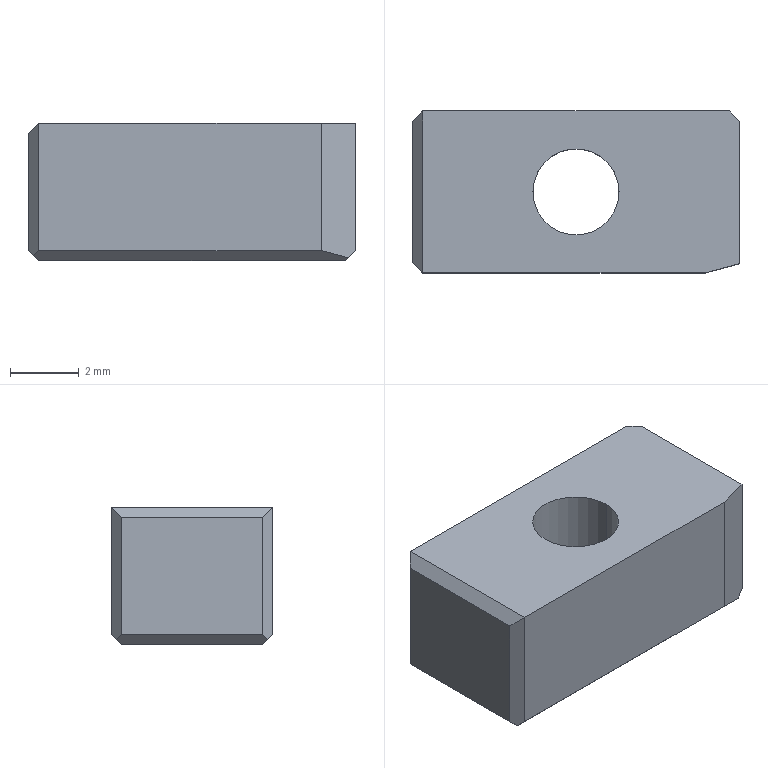Part | NX | 1 solid | 19 faces | box 9.5 x 4.7 x 4 mm | volume 156.004 mm3 | plane 15 | cylinder 2 | cone 2 | commonest cylinder face diameters 2.5 x2
STEP:
#1=CARTESIAN_POINT('',(-47.81,-38.329,4.403));
#2=VERTEX_POINT('',#1);
#3=CARTESIAN_POINT('',(-47.81,-38.329,0.7031));
#4=VERTEX_POINT('',#3);
#5=CARTESIAN_POINT('',(-47.81,-38.329,2.553));
#6=DIRECTION('',(0.,0.,-1.));
#7=VECTOR('',#6,1000.);
#8=LINE('',#5,#7);
#9=EDGE_CURVE('',#2,#4,#8,.T.);
#10=ORIENTED_EDGE('',*,*,#9,.T.);
#11=CARTESIAN_POINT('',(-39.61,-38.329,0.7031));
#12=VERTEX_POINT('',#11);
#13=CARTESIAN_POINT('',(-41.256,-38.329,0.7031));
#14=DIRECTION('',(-1.,0.,0.));
#15=VECTOR('',#14,1000.);
#16=LINE('',#13,#15);
#17=EDGE_CURVE('',#12,#4,#16,.T.);
#18=ORIENTED_EDGE('',*,*,#17,.F.);
#19=CARTESIAN_POINT('',(-39.61,-38.329,4.403));
#20=VERTEX_POINT('',#19);
#21=CARTESIAN_POINT('',(-39.61,-38.329,3.403));
#22=DIRECTION('',(0.,0.,-1.));
#23=VECTOR('',#22,1000.);
#24=LINE('',#21,#23);
#25=EDGE_CURVE('',#20,#12,#24,.T.);
#26=ORIENTED_EDGE('',*,*,#25,.F.);
#27=CARTESIAN_POINT('',(-41.256,-38.329,4.403));
#28=DIRECTION('',(1.,0.,0.));
#29=VECTOR('',#28,1000.);
#30=LINE('',#27,#29);
#31=EDGE_CURVE('',#2,#20,#30,.T.);
#32=ORIENTED_EDGE('',*,*,#31,.F.);
#33=EDGE_LOOP('',(#10,#18,#26,#32));
#34=FACE_BOUND('',#33,.T.);
#35=CARTESIAN_POINT('',(-48.11,-38.329,3.403));
#36=DIRECTION('',(0.,-1.,0.));
#37=DIRECTION('',(-1.,0.,0.));
#38=AXIS2_PLACEMENT_3D('',#35,#36,#37);
#39=PLANE('',#38);
#40=ADVANCED_FACE('',(#34),#39,.T.);
#41=CARTESIAN_POINT('',(-48.11,-33.929,4.103));
#42=VERTEX_POINT('',#41);
#43=CARTESIAN_POINT('',(-48.11,-33.929,0.7031));
#44=VERTEX_POINT('',#43);
#45=CARTESIAN_POINT('',(-48.11,-33.929,2.553));
#46=DIRECTION('',(0.,0.,-1.));
#47=VECTOR('',#46,1000.);
#48=LINE('',#45,#47);
#49=EDGE_CURVE('',#42,#44,#48,.T.);
#50=ORIENTED_EDGE('',*,*,#49,.T.);
#51=CARTESIAN_POINT('',(-48.11,-38.029,0.7031));
#52=VERTEX_POINT('',#51);
#53=CARTESIAN_POINT('',(-48.11,-35.979,0.7031));
#54=DIRECTION('',(0.,1.,0.));
#55=VECTOR('',#54,1000.);
#56=LINE('',#53,#55);
#57=EDGE_CURVE('',#52,#44,#56,.T.);
#58=ORIENTED_EDGE('',*,*,#57,.F.);
#59=CARTESIAN_POINT('',(-48.11,-38.029,4.103));
#60=VERTEX_POINT('',#59);
#61=CARTESIAN_POINT('',(-48.11,-38.029,2.553));
#62=DIRECTION('',(0.,0.,-1.));
#63=VECTOR('',#62,1000.);
#64=LINE('',#61,#63);
#65=EDGE_CURVE('',#60,#52,#64,.T.);
#66=ORIENTED_EDGE('',*,*,#65,.F.);
#67=CARTESIAN_POINT('',(-48.11,-35.979,4.103));
#68=DIRECTION('',(0.,-1.,0.));
#69=VECTOR('',#68,1000.);
#70=LINE('',#67,#69);
#71=EDGE_CURVE('',#42,#60,#70,.T.);
#72=ORIENTED_EDGE('',*,*,#71,.F.);
#73=EDGE_LOOP('',(#50,#58,#66,#72));
#74=FACE_BOUND('',#73,.T.);
#75=CARTESIAN_POINT('',(-48.11,-31.629,3.403));
#76=DIRECTION('',(-1.,0.,0.));
#77=DIRECTION('',(0.,1.,0.));
#78=AXIS2_PLACEMENT_3D('',#75,#76,#77);
#79=PLANE('',#78);
#80=ADVANCED_FACE('',(#74),#79,.T.);
#81=CARTESIAN_POINT('',(-47.81,-33.629,4.403));
#82=VERTEX_POINT('',#81);
#83=CARTESIAN_POINT('',(-47.81,-33.629,0.7031));
#84=VERTEX_POINT('',#83);
#85=CARTESIAN_POINT('',(-47.81,-33.629,2.553));
#86=DIRECTION('',(0.,0.,-1.));
#87=VECTOR('',#86,1000.);
#88=LINE('',#85,#87);
#89=EDGE_CURVE('',#82,#84,#88,.T.);
#90=ORIENTED_EDGE('',*,*,#89,.F.);
#91=CARTESIAN_POINT('',(-38.91,-33.629,4.403));
#92=VERTEX_POINT('',#91);
#93=CARTESIAN_POINT('',(-41.256,-33.629,4.403));
#94=DIRECTION('',(-1.,0.,0.));
#95=VECTOR('',#94,1000.);
#96=LINE('',#93,#95);
#97=EDGE_CURVE('',#92,#82,#96,.T.);
#98=ORIENTED_EDGE('',*,*,#97,.F.);
#99=CARTESIAN_POINT('',(-38.91,-33.629,0.7031));
#100=VERTEX_POINT('',#99);
#101=CARTESIAN_POINT('',(-38.91,-33.629,3.403));
#102=DIRECTION('',(0.,0.,1.));
#103=VECTOR('',#102,1000.);
#104=LINE('',#101,#103);
#105=EDGE_CURVE('',#100,#92,#104,.T.);
#106=ORIENTED_EDGE('',*,*,#105,.F.);
#107=CARTESIAN_POINT('',(-41.256,-33.629,0.7031));
#108=DIRECTION('',(1.,0.,0.));
#109=VECTOR('',#108,1000.);
#110=LINE('',#107,#109);
#111=EDGE_CURVE('',#84,#100,#110,.T.);
#112=ORIENTED_EDGE('',*,*,#111,.F.);
#113=EDGE_LOOP('',(#90,#98,#106,#112));
#114=FACE_BOUND('',#113,.T.);
#115=CARTESIAN_POINT('',(-38.61,-33.629,3.403));
#116=DIRECTION('',(0.,1.,0.));
#117=DIRECTION('',(1.,0.,0.));
#118=AXIS2_PLACEMENT_3D('',#115,#116,#117);
#119=PLANE('',#118);
#120=ADVANCED_FACE('',(#114),#119,.T.);
#121=CARTESIAN_POINT('',(-38.61,-33.929,0.7031));
#122=VERTEX_POINT('',#121);
#123=CARTESIAN_POINT('',(-38.61,-33.929,4.403));
#124=VERTEX_POINT('',#123);
#125=CARTESIAN_POINT('',(-38.61,-33.929,3.403));
#126=DIRECTION('',(0.,0.,1.));
#127=VECTOR('',#126,1000.);
#128=LINE('',#125,#127);
#129=EDGE_CURVE('',#122,#124,#128,.T.);
#130=ORIENTED_EDGE('',*,*,#129,.T.);
#131=CARTESIAN_POINT('',(-38.61,-38.061,4.403));
#132=VERTEX_POINT('',#131);
#133=CARTESIAN_POINT('',(-38.61,-36.022,4.403));
#134=DIRECTION('',(0.,1.,0.));
#135=VECTOR('',#134,1000.);
#136=LINE('',#133,#135);
#137=EDGE_CURVE('',#132,#124,#136,.T.);
#138=ORIENTED_EDGE('',*,*,#137,.F.);
#139=CARTESIAN_POINT('',(-38.61,-38.061,0.7031));
#140=VERTEX_POINT('',#139);
#141=CARTESIAN_POINT('',(-38.61,-38.061,3.403));
#142=DIRECTION('',(0.,0.,-1.));
#143=VECTOR('',#142,1000.);
#144=LINE('',#141,#143);
#145=EDGE_CURVE('',#132,#140,#144,.T.);
#146=ORIENTED_EDGE('',*,*,#145,.T.);
#147=CARTESIAN_POINT('',(-38.61,-36.022,0.7031));
#148=DIRECTION('',(0.,1.,0.));
#149=VECTOR('',#148,1000.);
#150=LINE('',#147,#149);
#151=EDGE_CURVE('',#140,#122,#150,.T.);
#152=ORIENTED_EDGE('',*,*,#151,.T.);
#153=EDGE_LOOP('',(#130,#138,#146,#152));
#154=FACE_BOUND('',#153,.T.);
#155=CARTESIAN_POINT('',(-38.61,-38.329,3.403));
#156=DIRECTION('',(1.,0.,0.));
#157=DIRECTION('',(0.,0.,1.));
#158=AXIS2_PLACEMENT_3D('',#155,#156,#157);
#159=PLANE('',#158);
#160=ADVANCED_FACE('',(#154),#159,.T.);
#161=ORIENTED_EDGE('',*,*,#25,.T.);
#162=CARTESIAN_POINT('',(-38.822,-38.118,0.4918));
#163=VERTEX_POINT('',#162);
#164=CARTESIAN_POINT('',(-41.256,-38.77,1.144));
#165=DIRECTION('',(0.9351,0.2506,-0.2506));
#166=VECTOR('',#165,1000.);
#167=LINE('',#164,#166);
#168=EDGE_CURVE('',#12,#163,#167,.T.);
#169=ORIENTED_EDGE('',*,*,#168,.T.);
#170=CARTESIAN_POINT('',(-35.91,-37.338,3.403));
#171=DIRECTION('',(-0.6947,-0.1862,-0.6947));
#172=VECTOR('',#171,1000.);
#173=LINE('',#170,#172);
#174=EDGE_CURVE('',#140,#163,#173,.T.);
#175=ORIENTED_EDGE('',*,*,#174,.F.);
#176=ORIENTED_EDGE('',*,*,#145,.F.);
#177=CARTESIAN_POINT('',(-41.256,-38.77,4.403));
#178=DIRECTION('',(-0.9659,-0.2588,0.));
#179=VECTOR('',#178,1000.);
#180=LINE('',#177,#179);
#181=EDGE_CURVE('',#132,#20,#180,.T.);
#182=ORIENTED_EDGE('',*,*,#181,.T.);
#183=EDGE_LOOP('',(#161,#169,#175,#176,#182));
#184=FACE_BOUND('',#183,.T.);
#185=CARTESIAN_POINT('',(-39.11,-38.195,1.903));
#186=DIRECTION('',(-0.2588,0.9659,0.));
#187=DIRECTION('',(0.,0.,1.));
#188=AXIS2_PLACEMENT_3D('',#185,#186,#187);
#189=PLANE('',#188);
#190=ADVANCED_FACE('',(#184),#189,.F.);
#191=ORIENTED_EDGE('',*,*,#105,.T.);
#192=CARTESIAN_POINT('',(-36.517,-36.022,4.403));
#193=DIRECTION('',(0.7071,-0.7071,0.));
#194=VECTOR('',#193,1000.);
#195=LINE('',#192,#194);
#196=EDGE_CURVE('',#92,#124,#195,.T.);
#197=ORIENTED_EDGE('',*,*,#196,.T.);
#198=ORIENTED_EDGE('',*,*,#129,.F.);
#199=CARTESIAN_POINT('',(-38.76,-33.779,0.5531));
#200=VERTEX_POINT('',#199);
#201=CARTESIAN_POINT('',(-36.517,-36.022,2.796));
#202=DIRECTION('',(-0.5774,0.5774,-0.5774));
#203=VECTOR('',#202,1000.);
#204=LINE('',#201,#203);
#205=EDGE_CURVE('',#122,#200,#204,.T.);
#206=ORIENTED_EDGE('',*,*,#205,.T.);
#207=CARTESIAN_POINT('',(-36.517,-36.022,-1.69));
#208=DIRECTION('',(-0.5774,0.5774,0.5774));
#209=VECTOR('',#208,1000.);
#210=LINE('',#207,#209);
#211=EDGE_CURVE('',#200,#100,#210,.T.);
#212=ORIENTED_EDGE('',*,*,#211,.T.);
#213=EDGE_LOOP('',(#191,#197,#198,#206,#212));
#214=FACE_BOUND('',#213,.T.);
#215=CARTESIAN_POINT('',(-38.76,-33.779,2.053));
#216=DIRECTION('',(-0.7071,-0.7071,0.));
#217=DIRECTION('',(-0.7071,0.7071,0.));
#218=AXIS2_PLACEMENT_3D('',#215,#216,#217);
#219=PLANE('',#218);
#220=ADVANCED_FACE('',(#214),#219,.F.);
#221=ORIENTED_EDGE('',*,*,#49,.F.);
#222=CARTESIAN_POINT('',(-48.81,-34.629,3.403));
#223=DIRECTION('',(0.5774,0.5774,0.5774));
#224=VECTOR('',#223,1000.);
#225=LINE('',#222,#224);
#226=EDGE_CURVE('',#42,#82,#225,.T.);
#227=ORIENTED_EDGE('',*,*,#226,.T.);
#228=ORIENTED_EDGE('',*,*,#89,.T.);
#229=CARTESIAN_POINT('',(-47.96,-33.779,0.5531));
#230=VERTEX_POINT('',#229);
#231=CARTESIAN_POINT('',(-41.256,-27.074,7.258));
#232=DIRECTION('',(-0.5774,-0.5774,-0.5774));
#233=VECTOR('',#232,1000.);
#234=LINE('',#231,#233);
#235=EDGE_CURVE('',#84,#230,#234,.T.);
#236=ORIENTED_EDGE('',*,*,#235,.T.);
#237=CARTESIAN_POINT('',(-50.81,-36.629,3.403));
#238=DIRECTION('',(-0.5774,-0.5774,0.5774));
#239=VECTOR('',#238,1000.);
#240=LINE('',#237,#239);
#241=EDGE_CURVE('',#230,#44,#240,.T.);
#242=ORIENTED_EDGE('',*,*,#241,.T.);
#243=EDGE_LOOP('',(#221,#227,#228,#236,#242));
#244=FACE_BOUND('',#243,.T.);
#245=CARTESIAN_POINT('',(-47.96,-33.779,2.553));
#246=DIRECTION('',(-0.7071,0.7071,0.));
#247=DIRECTION('',(0.,0.,1.));
#248=AXIS2_PLACEMENT_3D('',#245,#246,#247);
#249=PLANE('',#248);
#250=ADVANCED_FACE('',(#244),#249,.T.);
#251=ORIENTED_EDGE('',*,*,#9,.F.);
#252=CARTESIAN_POINT('',(-48.81,-37.329,3.403));
#253=DIRECTION('',(-0.5774,0.5774,-0.5774));
#254=VECTOR('',#253,1000.);
#255=LINE('',#252,#254);
#256=EDGE_CURVE('',#2,#60,#255,.T.);
#257=ORIENTED_EDGE('',*,*,#256,.T.);
#258=ORIENTED_EDGE('',*,*,#65,.T.);
#259=CARTESIAN_POINT('',(-47.96,-38.179,0.5531));
#260=VERTEX_POINT('',#259);
#261=CARTESIAN_POINT('',(-50.117,-36.022,2.71));
#262=DIRECTION('',(0.5774,-0.5774,-0.5774));
#263=VECTOR('',#262,1000.);
#264=LINE('',#261,#263);
#265=EDGE_CURVE('',#52,#260,#264,.T.);
#266=ORIENTED_EDGE('',*,*,#265,.T.);
#267=CARTESIAN_POINT('',(-45.11,-41.029,3.403));
#268=DIRECTION('',(0.5774,-0.5774,0.5774));
#269=VECTOR('',#268,1000.);
#270=LINE('',#267,#269);
#271=EDGE_CURVE('',#260,#4,#270,.T.);
#272=ORIENTED_EDGE('',*,*,#271,.T.);
#273=EDGE_LOOP('',(#251,#257,#258,#266,#272));
#274=FACE_BOUND('',#273,.T.);
#275=CARTESIAN_POINT('',(-47.96,-38.179,2.553));
#276=DIRECTION('',(-0.7071,-0.7071,0.));
#277=DIRECTION('',(-0.7071,0.7071,0.));
#278=AXIS2_PLACEMENT_3D('',#275,#276,#277);
#279=PLANE('',#278);
#280=ADVANCED_FACE('',(#274),#279,.T.);
#281=CARTESIAN_POINT('',(-47.81,-38.029,0.4031));
#282=VERTEX_POINT('',#281);
#283=CARTESIAN_POINT('',(-47.81,-33.929,0.4031));
#284=VERTEX_POINT('',#283);
#285=CARTESIAN_POINT('',(-47.81,-35.979,0.4031));
#286=DIRECTION('',(0.,1.,0.));
#287=VECTOR('',#286,1000.);
#288=LINE('',#285,#287);
#289=EDGE_CURVE('',#282,#284,#288,.T.);
#290=ORIENTED_EDGE('',*,*,#289,.T.);
#291=CARTESIAN_POINT('',(-38.91,-33.929,0.4031));
#292=VERTEX_POINT('',#291);
#293=CARTESIAN_POINT('',(-43.51,-33.929,0.4031));
#294=DIRECTION('',(1.,0.,0.));
#295=VECTOR('',#294,1000.);
#296=LINE('',#293,#295);
#297=EDGE_CURVE('',#284,#292,#296,.T.);
#298=ORIENTED_EDGE('',*,*,#297,.T.);
#299=CARTESIAN_POINT('',(-38.91,-38.029,0.4031));
#300=VERTEX_POINT('',#299);
#301=CARTESIAN_POINT('',(-38.91,-36.022,0.4031));
#302=DIRECTION('',(0.,1.,0.));
#303=VECTOR('',#302,1000.);
#304=LINE('',#301,#303);
#305=EDGE_CURVE('',#300,#292,#304,.T.);
#306=ORIENTED_EDGE('',*,*,#305,.F.);
#307=CARTESIAN_POINT('',(-43.86,-38.029,0.4031));
#308=DIRECTION('',(-1.,0.,0.));
#309=VECTOR('',#308,1000.);
#310=LINE('',#307,#309);
#311=EDGE_CURVE('',#300,#282,#310,.T.);
#312=ORIENTED_EDGE('',*,*,#311,.T.);
#313=EDGE_LOOP('',(#290,#298,#306,#312));
#314=FACE_BOUND('',#313,.T.);
#315=CARTESIAN_POINT('',(-45.06,-35.979,0.4031));
#316=VERTEX_POINT('',#315);
#317=CARTESIAN_POINT('',(-41.66,-35.979,0.4031));
#318=VERTEX_POINT('',#317);
#319=CARTESIAN_POINT('',(-43.36,-35.979,0.4031));
#320=DIRECTION('',(0.,0.,-1.));
#321=DIRECTION('',(-1.,0.,0.));
#322=AXIS2_PLACEMENT_3D('',#319,#320,#321);
#323=CIRCLE('',#322,1.7);
#324=EDGE_CURVE('',#316,#318,#323,.T.);
#325=ORIENTED_EDGE('',*,*,#324,.F.);
#326=CARTESIAN_POINT('',(-43.36,-35.979,0.4031));
#327=DIRECTION('',(0.,0.,-1.));
#328=DIRECTION('',(-1.,0.,0.));
#329=AXIS2_PLACEMENT_3D('',#326,#327,#328);
#330=CIRCLE('',#329,1.7);
#331=EDGE_CURVE('',#318,#316,#330,.T.);
#332=ORIENTED_EDGE('',*,*,#331,.F.);
#333=EDGE_LOOP('',(#325,#332));
#334=FACE_BOUND('',#333,.T.);
#335=CARTESIAN_POINT('',(-41.256,-36.022,0.4031));
#336=DIRECTION('',(0.,0.,-1.));
#337=DIRECTION('',(0.,-1.,0.));
#338=AXIS2_PLACEMENT_3D('',#335,#336,#337);
#339=PLANE('',#338);
#340=ADVANCED_FACE('',(#314,#334),#339,.T.);
#341=CARTESIAN_POINT('',(-42.11,-35.979,0.6629));
#342=VERTEX_POINT('',#341);
#343=CARTESIAN_POINT('',(-44.61,-35.979,0.6629));
#344=VERTEX_POINT('',#343);
#345=CARTESIAN_POINT('',(-43.36,-35.979,0.6629));
#346=DIRECTION('',(0.,0.,-1.));
#347=DIRECTION('',(-1.,0.,0.));
#348=AXIS2_PLACEMENT_3D('',#345,#346,#347);
#349=CIRCLE('',#348,1.25);
#350=EDGE_CURVE('',#342,#344,#349,.T.);
#351=ORIENTED_EDGE('',*,*,#350,.T.);
#352=CARTESIAN_POINT('',(-44.61,-35.979,4.403));
#353=VERTEX_POINT('',#352);
#354=CARTESIAN_POINT('',(-44.61,-35.979,0.4031));
#355=DIRECTION('',(0.,0.,-1.));
#356=VECTOR('',#355,1000.);
#357=LINE('',#354,#356);
#358=EDGE_CURVE('',#344,#353,#357,.F.);
#359=ORIENTED_EDGE('',*,*,#358,.T.);
#360=CARTESIAN_POINT('',(-42.11,-35.979,4.403));
#361=VERTEX_POINT('',#360);
#362=CARTESIAN_POINT('',(-43.36,-35.979,4.403));
#363=DIRECTION('',(0.,0.,-1.));
#364=DIRECTION('',(-1.,0.,0.));
#365=AXIS2_PLACEMENT_3D('',#362,#363,#364);
#366=CIRCLE('',#365,1.25);
#367=EDGE_CURVE('',#361,#353,#366,.T.);
#368=ORIENTED_EDGE('',*,*,#367,.F.);
#369=CARTESIAN_POINT('',(-42.11,-35.979,0.4031));
#370=DIRECTION('',(0.,0.,-1.));
#371=VECTOR('',#370,1000.);
#372=LINE('',#369,#371);
#373=EDGE_CURVE('',#342,#361,#372,.F.);
#374=ORIENTED_EDGE('',*,*,#373,.F.);
#375=EDGE_LOOP('',(#351,#359,#368,#374));
#376=FACE_BOUND('',#375,.T.);
#377=CARTESIAN_POINT('',(-43.36,-35.979,0.4031));
#378=DIRECTION('',(0.,0.,-1.));
#379=DIRECTION('',(-1.,0.,0.));
#380=AXIS2_PLACEMENT_3D('',#377,#378,#379);
#381=CYLINDRICAL_SURFACE('',#380,1.25);
#382=ADVANCED_FACE('',(#376),#381,.F.);
#383=ORIENTED_EDGE('',*,*,#350,.F.);
#384=CARTESIAN_POINT('',(-42.11,-35.979,0.6629));
#385=DIRECTION('',(0.866,0.,-0.5));
#386=VECTOR('',#385,1000.);
#387=LINE('',#384,#386);
#388=EDGE_CURVE('',#342,#318,#387,.T.);
#389=ORIENTED_EDGE('',*,*,#388,.T.);
#390=ORIENTED_EDGE('',*,*,#331,.T.);
#391=CARTESIAN_POINT('',(-44.61,-35.979,0.6629));
#392=DIRECTION('',(-0.866,0.,-0.5));
#393=VECTOR('',#392,1000.);
#394=LINE('',#391,#393);
#395=EDGE_CURVE('',#344,#316,#394,.T.);
#396=ORIENTED_EDGE('',*,*,#395,.F.);
#397=EDGE_LOOP('',(#383,#389,#390,#396));
#398=FACE_BOUND('',#397,.T.);
#399=CARTESIAN_POINT('',(-43.36,-35.979,0.6629));
#400=DIRECTION('',(0.,0.,-1.));
#401=DIRECTION('',(-1.,0.,0.));
#402=AXIS2_PLACEMENT_3D('',#399,#400,#401);
#403=CONICAL_SURFACE('',#402,1.25,1.047);
#404=ADVANCED_FACE('',(#398),#403,.F.);
#405=ORIENTED_EDGE('',*,*,#305,.T.);
#406=CARTESIAN_POINT('',(-35.91,-30.929,3.403));
#407=DIRECTION('',(0.5774,0.5774,0.5774));
#408=VECTOR('',#407,1000.);
#409=LINE('',#406,#408);
#410=EDGE_CURVE('',#292,#200,#409,.T.);
#411=ORIENTED_EDGE('',*,*,#410,.T.);
#412=ORIENTED_EDGE('',*,*,#205,.F.);
#413=ORIENTED_EDGE('',*,*,#151,.F.);
#414=ORIENTED_EDGE('',*,*,#174,.T.);
#415=CARTESIAN_POINT('',(-35.91,-41.029,3.403));
#416=DIRECTION('',(-0.5774,0.5774,-0.5774));
#417=VECTOR('',#416,1000.);
#418=LINE('',#415,#417);
#419=EDGE_CURVE('',#163,#300,#418,.T.);
#420=ORIENTED_EDGE('',*,*,#419,.T.);
#421=EDGE_LOOP('',(#405,#411,#412,#413,#414,#420));
#422=FACE_BOUND('',#421,.T.);
#423=CARTESIAN_POINT('',(-38.76,-34.845,0.5531));
#424=DIRECTION('',(-0.7071,0.,0.7071));
#425=DIRECTION('',(0.,1.,0.));
#426=AXIS2_PLACEMENT_3D('',#423,#424,#425);
#427=PLANE('',#426);
#428=ADVANCED_FACE('',(#422),#427,.F.);
#429=ORIENTED_EDGE('',*,*,#297,.F.);
#430=CARTESIAN_POINT('',(-45.717,-36.022,-1.69));
#431=DIRECTION('',(0.5774,-0.5774,-0.5774));
#432=VECTOR('',#431,1000.);
#433=LINE('',#430,#432);
#434=EDGE_CURVE('',#230,#284,#433,.T.);
#435=ORIENTED_EDGE('',*,*,#434,.F.);
#436=ORIENTED_EDGE('',*,*,#235,.F.);
#437=ORIENTED_EDGE('',*,*,#111,.T.);
#438=ORIENTED_EDGE('',*,*,#211,.F.);
#439=ORIENTED_EDGE('',*,*,#410,.F.);
#440=EDGE_LOOP('',(#429,#435,#436,#437,#438,#439));
#441=FACE_BOUND('',#440,.T.);
#442=CARTESIAN_POINT('',(-43.51,-33.779,0.5531));
#443=DIRECTION('',(0.,0.7071,-0.7071));
#444=DIRECTION('',(-1.,0.,0.));
#445=AXIS2_PLACEMENT_3D('',#442,#443,#444);
#446=PLANE('',#445);
#447=ADVANCED_FACE('',(#441),#446,.T.);
#448=ORIENTED_EDGE('',*,*,#17,.T.);
#449=ORIENTED_EDGE('',*,*,#271,.F.);
#450=CARTESIAN_POINT('',(-45.803,-36.022,-1.604));
#451=DIRECTION('',(-0.5774,-0.5774,0.5774));
#452=VECTOR('',#451,1000.);
#453=LINE('',#450,#452);
#454=EDGE_CURVE('',#282,#260,#453,.T.);
#455=ORIENTED_EDGE('',*,*,#454,.F.);
#456=ORIENTED_EDGE('',*,*,#311,.F.);
#457=ORIENTED_EDGE('',*,*,#419,.F.);
#458=ORIENTED_EDGE('',*,*,#168,.F.);
#459=EDGE_LOOP('',(#448,#449,#455,#456,#457,#458));
#460=FACE_BOUND('',#459,.T.);
#461=CARTESIAN_POINT('',(-43.86,-38.179,0.5531));
#462=DIRECTION('',(0.,-0.7071,-0.7071));
#463=DIRECTION('',(0.,-0.7071,0.7071));
#464=AXIS2_PLACEMENT_3D('',#461,#462,#463);
#465=PLANE('',#464);
#466=ADVANCED_FACE('',(#460),#465,.T.);
#467=ORIENTED_EDGE('',*,*,#289,.F.);
#468=ORIENTED_EDGE('',*,*,#454,.T.);
#469=ORIENTED_EDGE('',*,*,#265,.F.);
#470=ORIENTED_EDGE('',*,*,#57,.T.);
#471=ORIENTED_EDGE('',*,*,#241,.F.);
#472=ORIENTED_EDGE('',*,*,#434,.T.);
#473=EDGE_LOOP('',(#467,#468,#469,#470,#471,#472));
#474=FACE_BOUND('',#473,.T.);
#475=CARTESIAN_POINT('',(-47.96,-35.979,0.5531));
#476=DIRECTION('',(-0.7071,0.,-0.7071));
#477=DIRECTION('',(-0.7071,0.,0.7071));
#478=AXIS2_PLACEMENT_3D('',#475,#476,#477);
#479=PLANE('',#478);
#480=ADVANCED_FACE('',(#474),#479,.T.);
#481=CARTESIAN_POINT('',(-47.81,-35.979,4.403));
#482=DIRECTION('',(0.,-1.,0.));
#483=VECTOR('',#482,1000.);
#484=LINE('',#481,#483);
#485=EDGE_CURVE('',#82,#2,#484,.T.);
#486=ORIENTED_EDGE('',*,*,#485,.T.);
#487=ORIENTED_EDGE('',*,*,#31,.T.);
#488=ORIENTED_EDGE('',*,*,#181,.F.);
#489=ORIENTED_EDGE('',*,*,#137,.T.);
#490=ORIENTED_EDGE('',*,*,#196,.F.);
#491=ORIENTED_EDGE('',*,*,#97,.T.);
#492=EDGE_LOOP('',(#486,#487,#488,#489,#490,#491));
#493=FACE_BOUND('',#492,.T.);
#494=ORIENTED_EDGE('',*,*,#367,.T.);
#495=CARTESIAN_POINT('',(-43.36,-35.979,4.403));
#496=DIRECTION('',(0.,0.,-1.));
#497=DIRECTION('',(-1.,0.,0.));
#498=AXIS2_PLACEMENT_3D('',#495,#496,#497);
#499=CIRCLE('',#498,1.25);
#500=EDGE_CURVE('',#353,#361,#499,.T.);
#501=ORIENTED_EDGE('',*,*,#500,.T.);
#502=EDGE_LOOP('',(#494,#501));
#503=FACE_BOUND('',#502,.T.);
#504=CARTESIAN_POINT('',(-41.256,-36.022,4.403));
#505=DIRECTION('',(0.,0.,-1.));
#506=DIRECTION('',(0.,-1.,0.));
#507=AXIS2_PLACEMENT_3D('',#504,#505,#506);
#508=PLANE('',#507);
#509=ADVANCED_FACE('',(#493,#503),#508,.F.);
#510=ORIENTED_EDGE('',*,*,#485,.F.);
#511=ORIENTED_EDGE('',*,*,#226,.F.);
#512=ORIENTED_EDGE('',*,*,#71,.T.);
#513=ORIENTED_EDGE('',*,*,#256,.F.);
#514=EDGE_LOOP('',(#510,#511,#512,#513));
#515=FACE_BOUND('',#514,.T.);
#516=CARTESIAN_POINT('',(-47.96,-35.979,4.253));
#517=DIRECTION('',(-0.7071,0.,0.7071));
#518=DIRECTION('',(0.,1.,0.));
#519=AXIS2_PLACEMENT_3D('',#516,#517,#518);
#520=PLANE('',#519);
#521=ADVANCED_FACE('',(#515),#520,.T.);
#522=ORIENTED_EDGE('',*,*,#324,.T.);
#523=ORIENTED_EDGE('',*,*,#388,.F.);
#524=CARTESIAN_POINT('',(-43.36,-35.979,0.6629));
#525=DIRECTION('',(0.,0.,-1.));
#526=DIRECTION('',(-1.,0.,0.));
#527=AXIS2_PLACEMENT_3D('',#524,#525,#526);
#528=CIRCLE('',#527,1.25);
#529=EDGE_CURVE('',#344,#342,#528,.T.);
#530=ORIENTED_EDGE('',*,*,#529,.F.);
#531=ORIENTED_EDGE('',*,*,#395,.T.);
#532=EDGE_LOOP('',(#522,#523,#530,#531));
#533=FACE_BOUND('',#532,.T.);
#534=CARTESIAN_POINT('',(-43.36,-35.979,0.6629));
#535=DIRECTION('',(0.,0.,-1.));
#536=DIRECTION('',(-1.,0.,0.));
#537=AXIS2_PLACEMENT_3D('',#534,#535,#536);
#538=CONICAL_SURFACE('',#537,1.25,1.047);
#539=ADVANCED_FACE('',(#533),#538,.F.);
#540=ORIENTED_EDGE('',*,*,#358,.F.);
#541=ORIENTED_EDGE('',*,*,#529,.T.);
#542=ORIENTED_EDGE('',*,*,#373,.T.);
#543=ORIENTED_EDGE('',*,*,#500,.F.);
#544=EDGE_LOOP('',(#540,#541,#542,#543));
#545=FACE_BOUND('',#544,.T.);
#546=CARTESIAN_POINT('',(-43.36,-35.979,0.4031));
#547=DIRECTION('',(0.,0.,-1.));
#548=DIRECTION('',(-1.,0.,0.));
#549=AXIS2_PLACEMENT_3D('',#546,#547,#548);
#550=CYLINDRICAL_SURFACE('',#549,1.25);
#551=ADVANCED_FACE('',(#545),#550,.F.);
#552=CLOSED_SHELL('',(#40,#80,#120,#160,#190,#220,#250,#280,#340,#382,#404,#428,#447,#466,#480,#509,#521,#539,#551));
#553=MANIFOLD_SOLID_BREP('',#552);
#554=(LENGTH_UNIT()NAMED_UNIT(*)SI_UNIT(.MILLI.,.METRE.));
#555=UNCERTAINTY_MEASURE_WITH_UNIT(LENGTH_MEASURE(0.00001),#554,'','');
#556=(NAMED_UNIT(*)PLANE_ANGLE_UNIT()SI_UNIT($,.RADIAN.));
#557=(NAMED_UNIT(*)SI_UNIT($,.STERADIAN.)SOLID_ANGLE_UNIT());
#558=(GEOMETRIC_REPRESENTATION_CONTEXT(3)GLOBAL_UNCERTAINTY_ASSIGNED_CONTEXT((#555))GLOBAL_UNIT_ASSIGNED_CONTEXT((#554,#556,#557))REPRESENTATION_CONTEXT('',''));
#559=ADVANCED_BREP_SHAPE_REPRESENTATION('',(#553),#558);